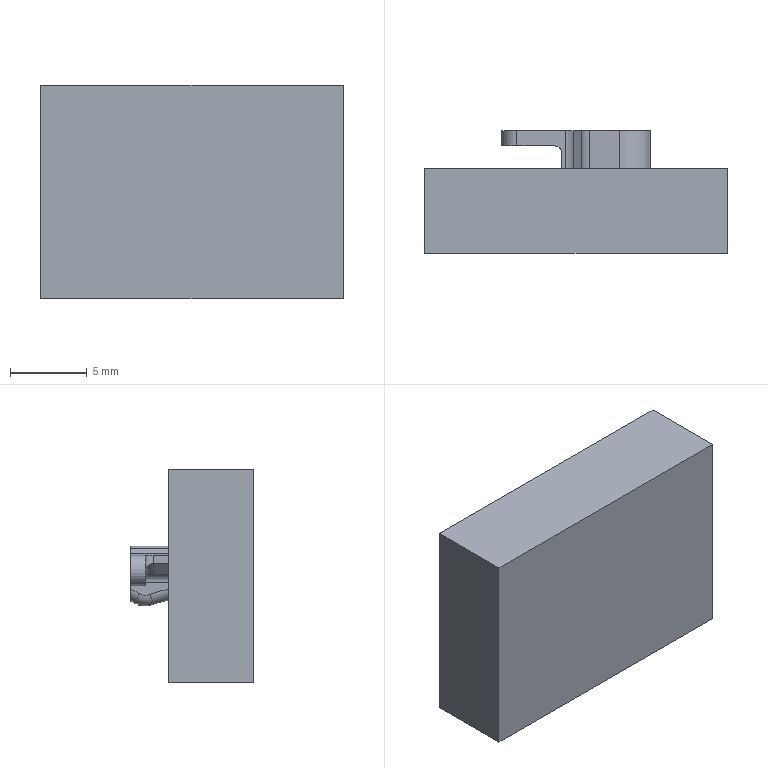NC program | NX | posted with a generic post | part box 19.7 x 8 x 13.91 mm
Lines 8250 to 9315 of 12456:
(FIXED_CONTOUR , TOOL : D2R0.5)
N16492 T09 M6
N16494 G54
N16496 G17 G0 G90 X-0.987 Y-3.274 B0. C0. S6500 M3
N16498 G43 Z30. H9
N16500 Z2.8
N16502 G94 G1 Z-1.531 F1000.
N16504 Y-3.17 Z-1.523
N16506 Y-3.085 Z-1.464
N16508 Y-3.063 Z-1.445 F1500.
N16510 X-0.989 Y-3.046 Z-1.453
N16512 X-0.99 Y-3.036 Z-1.464
N16514 X-0.992 Y-3.011 Z-1.476
N16516 X-0.997 Y-2.913 Z-1.5
N16518 Y-2.633 Z-1.35
N16520 Y-2.488 Z-1.278
N16522 Y-2.356 Z-1.216
N16524 Y-2.239 Z-1.179
N16526 Y-2.078 Z-1.166
N16528 Y-1.917 Z-1.169
N16530 Y-1.869 Z-1.181
N16532 Y-1.246 Z-1.38
N16534 Y-0.692 Z-1.501
N16536 Y-0.416 Z-1.536
N16538 Y0.133 Z-1.552
N16540 Y0.693 Z-1.501
N16542 Y1.07 Z-1.419
N16544 Y1.247 Z-1.377
N16546 Y1.918 Z-1.169
N16548 Y2.078 Z-1.165
N16550 Y2.239 Z-1.179
N16552 Y2.356 Z-1.215
N16554 Y2.495 Z-1.285
N16556 Y2.91 Z-1.499
N16558 X-0.987 Y3.064 Z-1.488
N16560 Y3.07 Z-1.501
N16562 X-0.986 Y3.076 Z-1.481
N16564 Y3.071 Z-1.464
N16566 X-0.99 Y2.984 Z-1.444
N16568 X-0.994 Y2.91 Z-1.443
N16570 Y2.633 Z-1.3
N16572 X-0.996 Y2.355 Z-1.163
N16574 X-0.995 Y2.219 Z-1.127
N16576 X-0.996 Y2.078 Z-1.115
N16578 X-0.995 Y1.927 Z-1.119
N16580 X-0.996 Y1.816 Z-1.149
N16582 X-0.994 Y1.247 Z-1.325
N16584 Y0.97 Z-1.389
N16586 Y0.693 Z-1.45
N16588 X-0.993 Y0.416 Z-1.477
N16590 X-0.994 Y0.139 Z-1.501
N16592 X-0.993 Y-0.139 Z-1.495
N16594 X-0.994 Y-0.416 Z-1.485
N16596 Y-0.693 Z-1.45
N16598 X-0.995 Y-1.216 Z-1.336
N16600 Y-1.247 Z-1.327
N16602 X-0.996 Y-1.818 Z-1.144
N16604 X-0.995 Y-1.914 Z-1.119
N16606 X-0.996 Y-2.09 Z-1.116
N16608 X-0.995 Y-2.219 Z-1.127
N16610 X-0.996 Y-2.359 Z-1.164
N16612 X-0.994 Y-2.633 Z-1.294
N16614 Y-2.91 Z-1.442
N16616 X-0.993 Y-2.925 Z-1.446
N16618 X-0.988 Y-2.997 Z-1.427
N16620 Y-3.003 Z-1.424
N16622 X-0.987 Y-3.015 Z-1.413
N16624 X-0.986 Y-3.025 Z-1.415
N16626 Y-3.066 Z-1.438
N16628 Y-3.087 Z-1.455
N16630 Y-3.066 Z-1.438
N16632 Y-3.025 Z-1.415
N16634 X-0.987 Y-3.015 Z-1.413
N16636 X-0.988 Y-3.003 Z-1.424
N16638 X-0.989 Y-2.986 Z-1.431
N16640 X-0.991 Y-2.959 Z-1.438
N16642 Y-2.633 Z-1.259
N16644 Y-2.464 Z-1.162
N16646 Y-2.41 Z-1.136
N16648 Y-2.356 Z-1.116
N16650 Y-2.301 Z-1.104
N16652 Y-2.247 Z-1.099
N16654 Y-2.078 Z-1.068
N16656 Y-2.024 Z-1.071
N16658 Y-1.97 Z-1.08
N16660 Y-1.801 Z-1.101
N16662 Y-1.692 Z-1.138
N16664 Y-1.524 Z-1.201
N16666 Y-1.415 Z-1.24
N16668 Y-1.247 Z-1.295
N16670 Y-0.97 Z-1.367
N16672 Y-0.693 Z-1.421
N16674 Y-0.416 Z-1.457
N16676 Y-0.139 Z-1.474
N16678 Y0.139
N16680 Y0.416 Z-1.457
N16682 Y0.693 Z-1.421
N16684 Y0.97 Z-1.367
N16686 Y1.247 Z-1.295
N16688 Y1.415 Z-1.24
N16690 Y1.524 Z-1.201
N16692 Y1.692 Z-1.138
N16694 Y1.801 Z-1.101
N16696 Y1.97 Z-1.08
N16698 Y2.024 Z-1.071
N16700 Y2.078 Z-1.068
N16702 Y2.247 Z-1.099
N16704 Y2.301 Z-1.104
N16706 Y2.356 Z-1.116
N16708 Y2.41 Z-1.136
N16710 Y2.464 Z-1.162
N16712 Y2.633 Z-1.259
N16714 Y2.97 Z-1.443
N16716 X-0.99 Y2.984 Z-1.444
N16718 X-0.986 Y3.071 Z-1.464
N16720 Y3.076 Z-1.481
N16722 Y3.078 Z-1.474
N16724 Y3.075 Z-1.463
N16726 Y3.036 Z-1.423
N16728 Y2.633 Z-1.202
N16730 Y2.563 Z-1.162
N16732 Y2.459 Z-1.111
N16734 Y2.356 Z-1.074
N16736 Y2.252 Z-1.051
N16738 Y2.148 Z-1.042
N16740 Y2.078 Z-1.029
N16742 Y1.975 Z-1.034
N16744 Y1.871 Z-1.052
N16746 Y1.801 Z-1.061
N16748 Y1.594 Z-1.131
N16750 Y1.317 Z-1.231
N16752 Y1.247 Z-1.254
N16754 Y0.97 Z-1.326
N16756 Y0.693 Z-1.381
N16758 Y0.416 Z-1.418
N16760 Y0.139 Z-1.435
N16762 Y-0.139
N16764 Y-0.416 Z-1.418
N16766 Y-0.693 Z-1.381
N16768 Y-0.97 Z-1.326
N16770 Y-1.247 Z-1.254
N16772 Y-1.317 Z-1.231
N16774 Y-1.594 Z-1.131
N16776 Y-1.801 Z-1.061
N16778 Y-1.871 Z-1.052
N16780 Y-1.975 Z-1.034
N16782 Y-2.078 Z-1.029
N16784 Y-2.148 Z-1.042
N16786 Y-2.252 Z-1.051
N16788 Y-2.356 Z-1.074
N16790 Y-2.459 Z-1.111
N16792 Y-2.563 Z-1.162
N16794 Y-2.633 Z-1.202
N16796 Y-2.995 Z-1.401
N16798 Y-3.012 Z-1.406
N16800 Y-3.066 Z-1.435
N16802 Y-3.088 Z-1.453
N16804 X-0.981 Y-3.099 Z-1.414
N16806 Y-3.083 Z-1.401
N16808 Y-2.633 Z-1.154
N16810 Y-2.5 Z-1.089
N16812 Y-2.356 Z-1.037
N16814 Y-2.211 Z-1.006
N16816 Y-2.078 Z-0.995
N16818 Y-1.934 Z-1.002
N16820 Y-1.801 Z-1.026
N16822 Y-1.524 Z-1.12
N16824 Y-1.235 Z-1.221
N16826 Y-0.97 Z-1.291
N16828 Y-0.693 Z-1.346
N16830 Y-0.416 Z-1.384
N16832 Y-0.139 Z-1.401
N16834 Y0.139
N16836 Y0.416 Z-1.384
N16838 Y0.693 Z-1.346
N16840 Y0.97 Z-1.291
N16842 Y1.247 Z-1.218
N16844 Y1.524 Z-1.12
N16846 Y1.801 Z-1.026
N16848 Y1.946 Z-1.001
N16850 Y2.078 Z-0.995
N16852 Y2.211 Z-1.006
N16854 Y2.356 Z-1.037
N16856 Y2.5 Z-1.089
N16858 Y2.633 Z-1.154
N16860 Y3.085 Z-1.402
N16862 Y3.096 Z-1.413
N16864 X-0.97 Y3.109 Z-1.365
N16866 Y3.017 Z-1.31
N16868 Y2.633 Z-1.1
N16870 Y2.544 Z-1.057
N16872 Y2.455 Z-1.025
N16874 Y2.356 Z-0.991
N16876 Y2.256 Z-0.978
N16878 Y2.167 Z-0.959
N16880 Y2.078 Z-0.952
N16882 Y1.99 Z-0.956
N16884 Y1.901 Z-0.971
N16886 Y1.801 Z-0.98
N16888 Y1.702 Z-1.011
N16890 Y1.524 Z-1.071
N16892 Y1.247 Z-1.17
N16894 Y1.147 Z-1.199
N16896 Y0.97 Z-1.246
N16898 Y0.693 Z-1.302
N16900 Y0.416 Z-1.339
N16902 Y0.139 Z-1.357
N16904 Y-0.139
N16906 Y-0.416 Z-1.339
N16908 Y-0.693 Z-1.302
N16910 Y-0.97 Z-1.246
N16912 Y-1.147 Z-1.199
N16914 Y-1.247 Z-1.17
N16916 Y-1.524 Z-1.071
N16918 Y-1.702 Z-1.011
N16920 Y-1.801 Z-0.98
N16922 Y-1.89 Z-0.964
N16924 Y-1.979 Z-0.96
N16926 Y-2.078 Z-0.952
N16928 Y-2.167 Z-0.959
N16930 Y-2.256 Z-0.978
N16932 Y-2.356 Z-0.991
N16934 Y-2.455 Z-1.025
N16936 Y-2.544 Z-1.057
N16938 Y-2.633 Z-1.1
N16940 Y-3.113 Z-1.362
N16942 X-0.959 Y-3.126 Z-1.315
N16944 Y-2.633 Z-1.046
N16946 Y-2.588 Z-1.024
N16948 Y-2.356 Z-0.945
N16950 Y-2.168 Z-0.921
N16952 Y-2.123 Z-0.911
N16954 Y-2.078 Z-0.907
N16956 Y-1.891 Z-0.924
N16958 Y-1.846 Z-0.926
N16960 Y-1.801 Z-0.934
N16962 Y-1.614 Z-0.992
N16964 Y-1.247 Z-1.123
N16966 Y-1.06 Z-1.176
N16968 Y-0.97 Z-1.2
N16970 Y-0.693 Z-1.256
N16972 Y-0.416 Z-1.295
N16974 Y-0.139 Z-1.313
N16976 Y0.139
N16978 Y0.416 Z-1.295
N16980 Y0.693 Z-1.256
N16982 Y0.97 Z-1.2
N16984 Y1.06 Z-1.176
N16986 Y1.247 Z-1.123
N16988 Y1.614 Z-0.992
N16990 Y1.801 Z-0.934
N16992 Y1.989 Z-0.917
N16994 Y2.034 Z-0.909
N16996 Y2.078 Z-0.907
N16998 Y2.123 Z-0.911
N17000 Y2.168 Z-0.921
N17002 Y2.356 Z-0.945
N17004 Y2.588 Z-1.024
N17006 Y2.633 Z-1.046
N17008 Y2.964 Z-1.226
N17010 Y3.122 Z-1.32
N17012 X-0.948 Y3.136 Z-1.276
N17014 Y2.911 Z-1.142
N17016 Y2.632 Z-0.991
N17018 Y2.356 Z-0.899
N17020 Y2.078 Z-0.863
N17022 Y1.801 Z-0.888
N17024 Y1.526 Z-0.974
N17026 Y1.247 Z-1.075
N17028 Y0.97 Z-1.154
N17030 Y0.693 Z-1.211
N17032 Y0.416 Z-1.25
N17034 Y0.139 Z-1.269
N17036 Y-0.139
N17038 Y-0.416 Z-1.25
N17040 Y-0.693 Z-1.211
N17042 Y-0.97 Z-1.154
N17044 Y-1.247 Z-1.075
N17046 Y-1.524 Z-0.975
N17048 Y-1.801 Z-0.888
N17050 Y-2.078 Z-0.863
N17052 Y-2.356 Z-0.899
N17054 Y-2.632 Z-0.991
N17056 Y-2.908 Z-1.14
N17058 Y-3.139 Z-1.269
N17060 X-0.934 Y-3.155 Z-1.227
N17062 Y-2.956 Z-1.124
N17064 Y-2.91 Z-1.095
N17066 Y-2.633 Z-0.945
N17068 Y-2.356 Z-0.854
N17070 Y-2.078 Z-0.819
N17072 Y-1.801 Z-0.843
N17074 Y-1.632 Z-0.895
N17076 Y-1.524 Z-0.927
N17078 Y-1.247 Z-1.028
N17080 Y-0.97 Z-1.108
N17082 Y-0.693 Z-1.166
N17084 Y-0.416 Z-1.206
N17086 Y-0.139 Z-1.225
N17088 Y0.139
N17090 Y0.416 Z-1.206
N17092 Y0.693 Z-1.166
N17094 Y0.97 Z-1.108
N17096 Y1.247 Z-1.028
N17098 Y1.524 Z-0.927
N17100 Y1.632 Z-0.896
N17102 Y1.801 Z-0.843
N17104 Y2.078 Z-0.819
N17106 Y2.356 Z-0.854
N17108 Y2.633 Z-0.945
N17110 Y2.91 Z-1.095
N17112 Y3.153 Z-1.23
N17114 X-0.92 Y3.167 Z-1.192
N17116 Y3.073 Z-1.14
N17118 Y2.855 Z-1.016
N17120 Y2.633 Z-0.897
N17122 Y2.356 Z-0.807
N17124 Y2.078 Z-0.774
N17126 Y1.801 Z-0.796
N17128 Y1.524 Z-0.877
N17130 Y1.247 Z-0.979
N17132 Y0.97 Z-1.061
N17134 Y0.693 Z-1.12
N17136 Y0.416 Z-1.16
N17138 Y0.139 Z-1.179
N17140 Y-0.139
N17142 Y-0.416 Z-1.16
N17144 Y-0.693 Z-1.12
N17146 Y-0.97 Z-1.061
N17148 Y-1.247 Z-0.979
N17150 Y-1.524 Z-0.877
N17152 Y-1.801 Z-0.796
N17154 Y-2.078 Z-0.774
N17156 Y-2.356 Z-0.807
N17158 Y-2.633 Z-0.897
N17160 Y-2.91 Z-1.046
N17162 Y-3.005 Z-1.106
N17164 Y-3.137 Z-1.175
N17166 Y-3.169 Z-1.189
N17168 X-0.903 Y-3.184 Z-1.147
N17170 Y-3.134 Z-1.124
N17172 Y-3.061 Z-1.086
N17174 Y-2.98 Z-1.035
N17176 Y-2.91 Z-1.
N17178 Y-2.67 Z-0.871
N17180 Y-2.633 Z-0.853
N17182 Y-2.393 Z-0.775
N17184 Y-2.356 Z-0.765
N17186 Y-2.078 Z-0.733
N17188 Y-1.801 Z-0.754
N17190 Y-1.524 Z-0.832
N17192 Y-1.247 Z-0.935
N17194 Y-0.97 Z-1.018
N17196 Y-0.693 Z-1.078
N17198 Y-0.416 Z-1.119
N17200 Y-0.139 Z-1.138
N17202 Y0.139
N17204 Y0.416 Z-1.119
N17206 Y0.693 Z-1.078
N17208 Y0.97 Z-1.018
N17210 Y1.247 Z-0.935
N17212 Y1.524 Z-0.832
N17214 Y1.801 Z-0.754
N17216 Y2.078 Z-0.733
N17218 Y2.356 Z-0.765
N17220 Y2.393 Z-0.775
N17222 Y2.633 Z-0.853
N17224 Y2.67 Z-0.871
N17226 Y3.117 Z-1.11
N17228 Y3.184 Z-1.148
N17230 X-0.886 Y3.199 Z-1.115
N17232 Y3.119 Z-1.07
N17234 Y2.738 Z-0.866
N17236 Y2.633 Z-0.815
N17238 Y2.461 Z-0.759
N17240 Y2.356 Z-0.729
N17242 Y2.078 Z-0.699
N17244 Y1.801 Z-0.719
N17246 Y1.696 Z-0.746
N17248 Y1.524 Z-0.795
N17250 Y1.247 Z-0.898
N17252 Y0.97 Z-0.982
N17254 Y0.693 Z-1.044
N17256 Y0.416 Z-1.084
N17258 Y0.139 Z-1.104
N17260 Y-0.139
N17262 Y-0.416 Z-1.084
N17264 Y-0.693 Z-1.044
N17266 Y-0.97 Z-0.982
N17268 Y-1.247 Z-0.898
N17270 Y-1.524 Z-0.795
N17272 Y-1.696 Z-0.746
N17274 Y-1.801 Z-0.719
N17276 Y-2.078 Z-0.699
N17278 Y-2.356 Z-0.729
N17280 Y-2.461 Z-0.759
N17282 Y-2.633 Z-0.815
N17284 Y-2.738 Z-0.866
N17286 Y-2.91 Z-0.959
N17288 Y-3.107 Z-1.057
N17290 Y-3.184 Z-1.102
N17292 Y-3.187 Z-1.108
N17294 Y-3.199 Z-1.116
N17296 X-0.865 Y-3.216 Z-1.08
N17298 Y-3.187 Z-1.063
N17300 Y-3.179 Z-1.046
N17302 Y-3.16 Z-1.034
N17304 Y-3.127 Z-1.022
N17306 Y-3.036 Z-0.972
N17308 Y-2.91 Z-0.909
N17310 Y-2.819 Z-0.86
N17312 Y-2.633 Z-0.769
N17314 Y-2.542 Z-0.74
N17316 Y-2.356 Z-0.687
N17318 Y-2.078 Z-0.659
N17320 Y-1.801 Z-0.678
N17322 Y-1.615 Z-0.725
N17324 Y-1.524 Z-0.751
N17326 Y-1.247 Z-0.855
N17328 Y-0.97 Z-0.94
N17330 Y-0.693 Z-1.002
N17332 Y-0.416 Z-1.044
N17334 Y-0.139 Z-1.064
N17336 Y0.139
N17338 Y0.416 Z-1.044
N17340 Y0.693 Z-1.002
N17342 Y0.97 Z-0.94
N17344 Y1.247 Z-0.855
N17346 Y1.524 Z-0.751
N17348 Y1.615 Z-0.725
N17350 Y1.801 Z-0.678
N17352 Y2.078 Z-0.659
N17354 Y2.356 Z-0.687
N17356 Y2.542 Z-0.74
N17358 Y2.633 Z-0.769
N17360 Y2.819 Z-0.86
N17362 Y3.021 Z-0.968
N17364 Y3.216 Z-1.08
N17366 X-0.844 Y3.234 Z-1.042
N17368 Y2.902 Z-0.854
N17370 Y2.625 Z-0.72
N17372 Y2.356 Z-0.644
N17374 Y2.078 Z-0.617
N17376 Y1.801 Z-0.636
N17378 Y1.524 Z-0.705
N17380 Y1.247 Z-0.809
N17382 Y0.97 Z-0.895
N17384 Y0.693 Z-0.96
N17386 Y0.416 Z-1.001
N17388 Y0.139 Z-1.022
N17390 Y-0.139
N17392 Y-0.416 Z-1.001
N17394 Y-0.7 Z-0.958
N17396 Y-0.97 Z-0.895
N17398 Y-1.247 Z-0.809
N17400 Y-1.532 Z-0.703
N17402 Y-1.801 Z-0.636
N17404 Y-2.078 Z-0.617
N17406 Y-2.356 Z-0.644
N17408 Y-2.633 Z-0.722
N17410 Y-2.92 Z-0.863
N17412 Y-3.122 Z-0.974
N17414 Y-3.159 Z-0.987
N17416 Y-3.18 Z-0.998
N17418 Y-3.187 Z-1.016
N17420 Y-3.234 Z-1.042
N17422 X-0.821 Y-3.253 Z-1.002
N17424 Y-3.187 Z-0.965
N17426 Y-3.184 Z-0.957
N17428 Y-2.91 Z-0.811
N17430 Y-2.716 Z-0.716
N17432 Y-2.633 Z-0.68
N17434 Y-2.55 Z-0.66
N17436 Y-2.356 Z-0.605
N17438 Y-2.078 Z-0.58
N17440 Y-1.801 Z-0.597
N17442 Y-1.607 Z-0.646
N17444 Y-1.524 Z-0.664
N17446 Y-1.247 Z-0.767
N17448 Y-1.164 Z-0.795
N17450 Y-0.97 Z-0.855
N17452 Y-0.693 Z-0.921
N17454 Y-0.416 Z-0.963
N17456 Y-0.139 Z-0.985
N17458 Y0.139
N17460 Y0.416 Z-0.963
N17462 Y0.693 Z-0.921
N17464 Y0.97 Z-0.855
N17466 Y1.164 Z-0.795
N17468 Y1.247 Z-0.767
N17470 Y1.524 Z-0.664
N17472 Y1.607 Z-0.646
N17474 Y1.801 Z-0.597
N17476 Y2.078 Z-0.58
N17478 Y2.356 Z-0.605
N17480 Y2.55 Z-0.66
N17482 Y2.633 Z-0.68
N17484 Y2.716 Z-0.716
N17486 Y2.91 Z-0.811
N17488 Y3.05 Z-0.887
N17490 Y3.253 Z-1.002
N17492 X-0.799 Y3.272 Z-0.962
N17494 Y2.91 Z-0.765
N17496 Y2.806 Z-0.714
N17498 Y2.633 Z-0.639
N17500 Y2.459 Z-0.596
N17502 Y2.356 Z-0.567
N17504 Y2.078 Z-0.543
N17506 Y1.801 Z-0.56
N17508 Y1.697 Z-0.586
N17510 Y1.524 Z-0.622
N17512 Y1.247 Z-0.725
N17514 Y1.074 Z-0.783
N17516 Y0.97 Z-0.815
N17518 Y0.693 Z-0.882
N17520 Y0.416 Z-0.925
N17522 Y0.139 Z-0.948
N17524 Y-0.139
N17526 Y-0.416 Z-0.925
N17528 Y-0.693 Z-0.882
N17530 Y-0.97 Z-0.815
N17532 Y-1.074 Z-0.783
N17534 Y-1.247 Z-0.725
N17536 Y-1.524 Z-0.622
N17538 Y-1.698 Z-0.586
N17540 Y-1.801 Z-0.56
N17542 Y-2.078 Z-0.543
N17544 Y-2.356 Z-0.567
N17546 Y-2.459 Z-0.596
N17548 Y-2.633 Z-0.639
N17550 Y-2.806 Z-0.714
N17552 Y-2.91 Z-0.765
N17554 Y-3.019 Z-0.823
N17556 Y-3.114 Z-0.881
N17558 Y-3.207 Z-0.925
N17560 Y-3.271 Z-0.962
N17562 X-0.774 Y-3.288 Z-0.927
N17564 Y-3.152 Z-0.857
N17566 Y-3.109 Z-0.837
N17568 Y-2.91 Z-0.716
N17570 Y-2.633 Z-0.596
N17572 Y-2.356 Z-0.526
N17574 Y-2.078 Z-0.504
N17576 Y-1.801 Z-0.521
N17578 Y-1.524 Z-0.579
N17580 Y-1.247 Z-0.681
N17582 Y-0.97 Z-0.773
N17584 Y-0.693 Z-0.842
N17586 Y-0.416 Z-0.886
N17588 Y-0.139 Z-0.909
N17590 Y0.139
N17592 Y0.416 Z-0.886
N17594 Y0.701 Z-0.84
N17596 Y0.978 Z-0.771
N17598 Y1.247 Z-0.681
N17600 Y1.524 Z-0.579
N17602 Y1.801 Z-0.521
N17604 Y2.078 Z-0.504
N17606 Y2.356 Z-0.526
N17608 Y2.633 Z-0.596
N17610 Y2.91 Z-0.716
N17612 Y3.187 Z-0.875
N17614 Y3.288 Z-0.927
N17616 X-0.747 Y3.304 Z-0.893
N17618 Y3.187 Z-0.831
N17620 Y3.008 Z-0.727
N17622 Y2.91 Z-0.675
N17624 Y2.731 Z-0.598
N17626 Y2.633 Z-0.559
N17628 Y2.356 Z-0.492
N17630 Y2.078 Z-0.47
N17632 Y1.801 Z-0.487
N17634 Y1.524 Z-0.543
N17636 Y1.345 Z-0.609
N17638 Y1.149 Z-0.678
N17640 Y0.97 Z-0.738
N17642 Y0.693 Z-0.807
N17644 Y0.416 Z-0.852
N17646 Y0.139 Z-0.875
N17648 Y-0.139
N17650 Y-0.416 Z-0.852
N17652 Y-0.693 Z-0.807
N17654 Y-0.97 Z-0.738
N17656 Y-1.149 Z-0.678
N17658 Y-1.345 Z-0.609
N17660 Y-1.524 Z-0.543
N17662 Y-1.801 Z-0.487
N17664 Y-2.078 Z-0.47
N17666 Y-2.356 Z-0.492
N17668 Y-2.633 Z-0.559
N17670 Y-2.731 Z-0.598
N17672 Y-2.91 Z-0.675
N17674 Y-2.976 Z-0.71
N17676 Y-3.104 Z-0.788
N17678 Y-3.232 Z-0.853
N17680 Y-3.304 Z-0.893
N17682 X-0.72 Y-3.322 Z-0.858
N17684 Y-3.099 Z-0.738
N17686 Y-3.048 Z-0.707
N17688 Y-2.91 Z-0.635
N17690 Y-2.839 Z-0.604
N17692 Y-2.633 Z-0.524
N17694 Y-2.356 Z-0.458
N17696 Y-2.078 Z-0.437
N17698 Y-1.801 Z-0.453
N17700 Y-1.524 Z-0.508
N17702 Y-1.454 Z-0.534
N17704 Y-1.247 Z-0.605
N17706 Y-1.04 Z-0.679
N17708 Y-0.97 Z-0.703
N17710 Y-0.693 Z-0.773
N17712 Y-0.416 Z-0.818
N17714 Y-0.139 Z-0.841
N17716 Y0.139
N17718 Y0.416 Z-0.818
N17720 Y0.693 Z-0.773
N17722 Y0.97 Z-0.703
N17724 Y1.04 Z-0.679
N17726 Y1.247 Z-0.605
N17728 Y1.454 Z-0.534
N17730 Y1.524 Z-0.508
N17732 Y1.801 Z-0.453
N17734 Y2.078 Z-0.437
N17736 Y2.356 Z-0.458
N17738 Y2.633 Z-0.524
N17740 Y2.839 Z-0.604
N17742 Y2.91 Z-0.635
N17744 Y3.116 Z-0.744
N17746 Y3.204 Z-0.794
N17748 Y3.322 Z-0.858
N17750 X-0.702 Y3.334 Z-0.836
N17752 X-0.69 Y3.339 Z-0.825
N17754 Y3.187 Z-0.74
N17756 Y2.91 Z-0.594
N17758 Y2.633 Z-0.485
N17760 Y2.405 Z-0.432
N17762 Y2.356 Z-0.424
N17764 Y2.078 Z-0.403
N17766 Y1.801 Z-0.419
N17768 Y1.752 Z-0.426
N17770 Y1.524 Z-0.471
N17772 Y1.222 Z-0.575
N17774 Y0.97 Z-0.666
N17776 Y0.693 Z-0.735
N17778 Y0.465 Z-0.773
N17780 Y0.416 Z-0.784
N17782 Y0.139 Z-0.807
N17784 Y-0.139
N17786 Y-0.416 Z-0.784
N17788 Y-0.465 Z-0.773
N17790 Y-0.693 Z-0.735
N17792 Y-0.97 Z-0.666
N17794 Y-1.297 Z-0.548
N17796 Y-1.524 Z-0.471
N17798 Y-1.752 Z-0.426
N17800 Y-1.801 Z-0.419
N17802 Y-2.078 Z-0.403
N17804 Y-2.356 Z-0.424
N17806 Y-2.405 Z-0.432
N17808 Y-2.633 Z-0.485
N17810 Y-2.91 Z-0.594
N17812 Y-3.104 Z-0.694
N17814 Y-3.34 Z-0.825
N17816 X-0.658 Y-3.355 Z-0.795
N17818 Y-3.285 Z-0.754
N17820 Y-3.125 Z-0.666
N17822 Y-2.91 Z-0.556
N17824 Y-2.633 Z-0.445
N17826 Y-2.532 Z-0.422
N17828 Y-2.444 Z-0.409
N17830 Y-2.356 Z-0.392
N17832 Y-2.078 Z-0.372
N17834 Y-1.801 Z-0.387
N17836 Y-1.625 Z-0.413
N17838 Y-1.524 Z-0.433
N17840 Y-1.247 Z-0.53
N17842 Y-0.97 Z-0.632
N17844 Y-0.793 Z-0.672
N17846 Y-0.693 Z-0.698
N17848 Y-0.592 Z-0.714
N17850 Y-0.416 Z-0.752
N17852 Y-0.139 Z-0.776
N17854 Y0.139
N17856 Y0.416 Z-0.752
N17858 Y0.592 Z-0.715
N17860 Y0.693 Z-0.698
N17862 Y0.793 Z-0.672
N17864 Y0.97 Z-0.632
N17866 Y1.424 Z-0.467
N17868 Y1.524 Z-0.433
N17870 Y1.625 Z-0.413
N17872 Y1.801 Z-0.387
N17874 Y2.078 Z-0.372
N17876 Y2.356 Z-0.392
N17878 Y2.444 Z-0.409
N17880 Y2.532 Z-0.422
N17882 Y2.633 Z-0.445
N17884 Y2.91 Z-0.556
N17886 Y2.998 Z-0.6
N17888 Y3.284 Z-0.754
N17890 Y3.355 Z-0.794
N17892 X-0.624 Y3.372 Z-0.762
N17894 Y3.187 Z-0.659
N17896 Y3.064 Z-0.594
N17898 Y2.91 Z-0.517
N17900 Y2.664 Z-0.418
N17902 Y2.633 Z-0.407
N17904 Y2.51 Z-0.389
N17906 Y2.356 Z-0.36
N17908 Y2.078 Z-0.339
N17910 Y1.801 Z-0.354
N17912 Y1.524 Z-0.396
N17914 Y1.493 Z-0.405
N17916 Y1.247 Z-0.493
N17918 Y0.97 Z-0.595
N17920 Y0.724 Z-0.652
N17922 Y0.693 Z-0.661
N17924 Y0.416 Z-0.719
N17926 Y0.139 Z-0.743
N17928 Y-0.139
N17930 Y-0.416 Z-0.719
N17932 Y-0.693 Z-0.661
N17934 Y-0.724 Z-0.652
N17936 Y-0.97 Z-0.595
N17938 Y-1.493 Z-0.405
N17940 Y-1.524 Z-0.396
N17942 Y-1.801 Z-0.354
N17944 Y-2.078 Z-0.339
N17946 Y-2.356 Z-0.36
N17948 Y-2.51 Z-0.389
N17950 Y-2.633 Z-0.407
N17952 Y-2.664 Z-0.418
N17954 Y-2.91 Z-0.517
N17956 Y-3.146 Z-0.637
N17958 Y-3.372 Z-0.762
N17960 X-0.59 Y-3.391 Z-0.731
N17962 Y-3.131 Z-0.588
N17964 Y-2.91 Z-0.477
N17966 Y-2.797 Z-0.432
N17968 Y-2.633 Z-0.377
N17970 Y-2.577 Z-0.369
N17972 Y-2.356 Z-0.326
N17974 Y-2.078 Z-0.307
N17976 Y-1.801 Z-0.321
N17978 Y-1.689 Z-0.338
N17980 Y-1.524 Z-0.366
N17982 Y-1.469 Z-0.384
N17984 Y-1.36 Z-0.416
N17986 Y-0.97 Z-0.559
N17988 Y-0.858 Z-0.585
N17990 Y-0.693 Z-0.631
N17992 Y-0.528 Z-0.661
N17994 Y-0.416 Z-0.685
N17996 Y-0.139 Z-0.71
N17998 Y0.139
N18000 Y0.416 Z-0.685
N18002 Y0.528 Z-0.661
N18004 Y0.693 Z-0.631
N18006 Y0.858 Z-0.585
N18008 Y0.97 Z-0.559
N18010 Y1.359 Z-0.416
N18012 Y1.469 Z-0.384
N18014 Y1.524 Z-0.366
N18016 Y1.689 Z-0.338
N18018 Y1.801 Z-0.321
N18020 Y2.078 Z-0.307
N18022 Y2.356 Z-0.326
N18024 Y2.576 Z-0.369
N18026 Y2.633 Z-0.377
N18028 Y2.797 Z-0.432
N18030 Y2.91 Z-0.477
N18032 Y3.187 Z-0.617
N18034 Y3.391 Z-0.731
N18036 X-0.568 Y3.404 Z-0.709
N18038 X-0.556 Y3.409 Z-0.701
N18040 Y3.187 Z-0.577
N18042 Y2.91 Z-0.439
N18044 Y2.633 Z-0.347
N18046 Y2.356 Z-0.294
N18048 Y2.078 Z-0.275
N18050 Y1.789 Z-0.29
N18052 Y1.512 Z-0.34
N18054 Y1.424 Z-0.368
N18056 Y1.235 Z-0.424
N18058 Y0.958 Z-0.526
N18060 Y0.681 Z-0.604
N18062 Y0.404 Z-0.653
N18064 Y0.139 Z-0.677
N18066 Y-0.139
N18068 Y-0.416 Z-0.652
N18070 Y-0.693 Z-0.601
N18072 Y-0.97 Z-0.523
N18074 Y-1.247 Z-0.419
N18076 Y-1.424 Z-0.368
N18078 Y-1.524 Z-0.336
N18080 Y-1.801 Z-0.289
N18082 Y-2.078 Z-0.275
N18084 Y-2.368 Z-0.296
N18086 Y-2.645 Z-0.35
N18088 Y-2.91 Z-0.439
N18090 Y-3.2 Z-0.584
N18092 Y-3.409 Z-0.701
N18094 X-0.518 Y-3.426 Z-0.673
N18096 Y-3.187 Z-0.541
N18098 Y-2.997 Z-0.446
N18100 Y-2.91 Z-0.406
N18102 Y-2.72 Z-0.343
N18104 Y-2.633 Z-0.317
N18106 Y-2.443 Z-0.281
N18108 Y-2.356 Z-0.266
N18110 Y-2.078 Z-0.247
N18112 Y-1.801 Z-0.26
N18114 Y-1.714 Z-0.273
N18116 Y-1.524 Z-0.306
N18118 Y-1.437 Z-0.33
N18120 Y-1.374 Z-0.351
N18122 Y-1.247 Z-0.388
N18124 Y-0.97 Z-0.49
N18126 Y-0.883 Z-0.516
N18128 Y-0.693 Z-0.57
N18130 Y-0.606 Z-0.588
N18132 Y-0.416 Z-0.623
N18134 Y-0.139 Z-0.649
N18136 Y0.139
N18138 Y0.416 Z-0.623
N18140 Y0.606 Z-0.588
N18142 Y0.693 Z-0.57
N18144 Y0.883 Z-0.516
N18146 Y0.97 Z-0.49
N18148 Y1.247 Z-0.388
N18150 Y1.374 Z-0.351
N18152 Y1.437 Z-0.33
N18154 Y1.524 Z-0.306
N18156 Y1.714 Z-0.273
N18158 Y1.801 Z-0.26
N18160 Y2.078 Z-0.247
N18162 Y2.356 Z-0.266
N18164 Y2.443 Z-0.281
N18166 Y2.633 Z-0.317
N18168 Y2.72 Z-0.343
N18170 Y2.91 Z-0.406
N18172 Y2.997 Z-0.446
N18174 Y3.187 Z-0.541
N18176 Y3.426 Z-0.673
N18178 X-0.48 Y3.443 Z-0.645
N18180 Y3.187 Z-0.505
N18182 Y3.072 Z-0.447
N18184 Y2.91 Z-0.374
N18186 Y2.794 Z-0.336
N18188 Y2.633 Z-0.287
N18190 Y2.517 Z-0.265
N18192 Y2.356 Z-0.238
N18194 Y2.078 Z-0.22
N18196 Y1.801 Z-0.232
N18198 Y1.64 Z-0.257
N18200 Y1.524 Z-0.276
N18202 Y1.362 Z-0.321
N18204 Y1.247 Z-0.356
N18206 Y0.97 Z-0.457
N18208 Y0.808 Z-0.506
N18210 Y0.693 Z-0.539
N18212 Y0.531 Z-0.572
N18214 Y0.416 Z-0.593
N18216 Y0.139 Z-0.621
N18218 Y-0.139
N18220 Y-0.416 Z-0.593
N18222 Y-0.531 Z-0.572
N18224 Y-0.693 Z-0.539
N18226 Y-0.808 Z-0.506
N18228 Y-0.97 Z-0.457
N18230 Y-1.247 Z-0.356
N18232 Y-1.362 Z-0.321
N18234 Y-1.524 Z-0.276
N18236 Y-1.64 Z-0.256
N18238 Y-1.801 Z-0.232
N18240 Y-2.078 Z-0.22
N18242 Y-2.356 Z-0.238
N18244 Y-2.517 Z-0.265
N18246 Y-2.633 Z-0.287
N18248 Y-2.794 Z-0.336
N18250 Y-2.91 Z-0.374
N18252 Y-3.072 Z-0.447
N18254 Y-3.187 Z-0.505
N18256 Y-3.443 Z-0.645
N18258 X-0.442 Y-3.462 Z-0.618
N18260 Y-3.187 Z-0.469
N18262 Y-3.146 Z-0.449
N18264 Y-2.91 Z-0.342
N18266 Y-2.633 Z-0.258
N18268 Y-2.356 Z-0.21
N18270 Y-2.078 Z-0.192
N18272 Y-1.801 Z-0.204
N18274 Y-1.524 Z-0.247
N18276 Y-1.247 Z-0.325
N18278 Y-0.97 Z-0.424
N18280 Y-0.693 Z-0.508
N18282 Y-0.416 Z-0.564
N18284 Y-0.139 Z-0.592
N18286 Y0.139
N18288 Y0.416 Z-0.564
N18290 Y0.693 Z-0.508
N18292 Y0.97 Z-0.424
N18294 Y1.247 Z-0.325
N18296 Y1.524 Z-0.247
N18298 Y1.801 Z-0.204
N18300 Y2.078 Z-0.192
N18302 Y2.356 Z-0.21
N18304 Y2.633 Z-0.258
N18306 Y2.91 Z-0.342
N18308 Y3.146 Z-0.449
N18310 Y3.187 Z-0.469
N18312 Y3.462 Z-0.618
N18314 X-0.42 Y3.473 Z-0.605
N18316 X-0.402 Y3.48 Z-0.596
N18318 Y3.187 Z-0.436
N18320 Y2.91 Z-0.312
N18322 Y2.633 Z-0.23
N18324 Y2.356 Z-0.184
N18326 Y2.078 Z-0.167
N18328 Y1.801 Z-0.178
N18330 Y1.524 Z-0.219
N18332 Y1.247 Z-0.296
N18334 Y0.931 Z-0.407
N18336 Y0.693 Z-0.48
N18338 Y0.416 Z-0.537
N18340 Y0.139 Z-0.567
N18342 Y-0.139
N18344 Y-0.416 Z-0.537
N18346 Y-0.693 Z-0.48
N18348 Y-0.97 Z-0.394
N18350 Y-1.247 Z-0.295
N18352 Y-1.524 Z-0.219
N18354 Y-1.801 Z-0.178
N18356 Y-2.078 Z-0.167
N18358 Y-2.356 Z-0.184
N18360 Y-2.633 Z-0.23
N18362 Y-2.91 Z-0.312
N18364 Y-3.187 Z-0.436
N18366 Y-3.48 Z-0.596
N18368 X-0.36 Y-3.498 Z-0.576
N18370 Y-3.309 Z-0.472
N18372 Y-3.187 Z-0.408
N18374 Y-3.032 Z-0.338
N18376 Y-2.91 Z-0.287
N18378 Y-2.755 Z-0.241
N18380 Y-2.633 Z-0.207
N18382 Y-2.356 Z-0.161
N18384 Y-2.078 Z-0.145
N18386 Y-1.801 Z-0.156
N18388 Y-1.524 Z-0.196
N18390 Y-1.402 Z-0.227
N18392 Y-1.247 Z-0.27
N18394 Y-0.97 Z-0.369
N18396 Y-0.848 Z-0.409
N18398 Y-0.693 Z-0.456
N18400 Y-0.416 Z-0.514
N18402 Y-0.139 Z-0.544
N18404 Y0.139
N18406 Y0.416 Z-0.514
N18408 Y0.693 Z-0.456
N18410 Y0.848 Z-0.409
N18412 Y0.97 Z-0.369
N18414 Y1.247 Z-0.27
N18416 Y1.402 Z-0.227
N18418 Y1.524 Z-0.196
N18420 Y1.801 Z-0.156
N18422 Y2.078 Z-0.145
N18424 Y2.356 Z-0.161
N18426 Y2.633 Z-0.207
N18428 Y2.755 Z-0.241
N18430 Y2.91 Z-0.287
N18432 Y3.032 Z-0.338
N18434 Y3.187 Z-0.408
N18436 Y3.309 Z-0.472
N18438 Y3.498 Z-0.576
N18440 X-0.318 Y3.516 Z-0.555
N18442 Y3.392 Z-0.487
N18444 Y3.187 Z-0.38
N18446 Y3.115 Z-0.347
N18448 Y2.91 Z-0.261
N18450 Y2.633 Z-0.183
N18452 Y2.356 Z-0.139
N18454 Y2.078 Z-0.123
N18456 Y1.801 Z-0.133
N18458 Y1.524 Z-0.172
N18460 Y1.247 Z-0.245
N18462 Y0.97 Z-0.343
N18464 Y0.693 Z-0.432
N18466 Y0.416 Z-0.492
N18468 Y0.139 Z-0.522
N18470 Y-0.139
N18472 Y-0.416 Z-0.492
N18474 Y-0.693 Z-0.432
N18476 Y-0.97 Z-0.343
N18478 Y-1.247 Z-0.245
N18480 Y-1.524 Z-0.172
N18482 Y-1.801 Z-0.133
N18484 Y-2.078 Z-0.123
N18486 Y-2.356 Z-0.139
N18488 Y-2.633 Z-0.183
N18490 Y-2.91 Z-0.261
N18492 Y-3.115 Z-0.347
N18494 Y-3.187 Z-0.38
N18496 Y-3.464 Z-0.526
N18498 Y-3.516 Z-0.555
N18500 X-0.276 Y-3.533 Z-0.535
N18502 Y-3.48 Z-0.505
N18504 Y-3.187 Z-0.352
N18506 Y-2.91 Z-0.237
N18508 Y-2.633 Z-0.161
N18510 Y-2.356 Z-0.117
N18512 Y-2.067 Z-0.102
N18514 Y-1.79 Z-0.113
N18516 Y-1.513 Z-0.152
N18518 Y-1.236 Z-0.224
N18520 Y-0.958 Z-0.322
N18522 Y-0.693 Z-0.409
N18524 Y-0.404 Z-0.471
N18526 Y-0.133 Z-0.501
N18528 Y0.139
N18530 Y0.416 Z-0.47
N18532 Y0.693 Z-0.409
N18534 Y0.958 Z-0.322
N18536 Y1.247 Z-0.22
N18538 Y1.524 Z-0.15
N18540 Y1.801 Z-0.111
N18542 Y2.09 Z-0.102
N18544 Y2.367 Z-0.118
N18546 Y2.644 Z-0.163
N18548 Y2.921 Z-0.241
N18550 Y3.201 Z-0.359
N18552 Y3.479 Z-0.504
N18554 Y3.533 Z-0.535
N18556 X-0.232 Y3.55 Z-0.516
N18558 Y3.187 Z-0.327
N18560 Y3.007 Z-0.251
N18562 Y2.91 Z-0.214
N18564 Y2.73 Z-0.165
N18566 Y2.633 Z-0.142
N18568 Y2.452 Z-0.113
N18570 Y2.356 Z-0.101
N18572 Y2.078 Z-0.087
N18574 Y1.801 Z-0.096
N18576 Y1.704 Z-0.107
N18578 Y1.524 Z-0.132
N18580 Y1.427 Z-0.152
N18582 Y1.247 Z-0.198
N18584 Y0.873 Z-0.33
N18586 Y0.693 Z-0.389
N18588 Y0.596 Z-0.413
N18590 Y0.416 Z-0.453
N18592 Y0.235 Z-0.473
N18594 Y0.139 Z-0.486
N18596 Y0.09 Z-0.488
N18598 Y-0.09
N18600 Y-0.139 Z-0.486
N18602 Y-0.319 Z-0.466
N18604 Y-0.416 Z-0.453
N18606 Y-0.513 Z-0.428
N18608 Y-0.693 Z-0.389
N18610 Y-0.873 Z-0.33
N18612 Y-1.247 Z-0.198
N18614 Y-1.427 Z-0.152
N18616 Y-1.524 Z-0.132